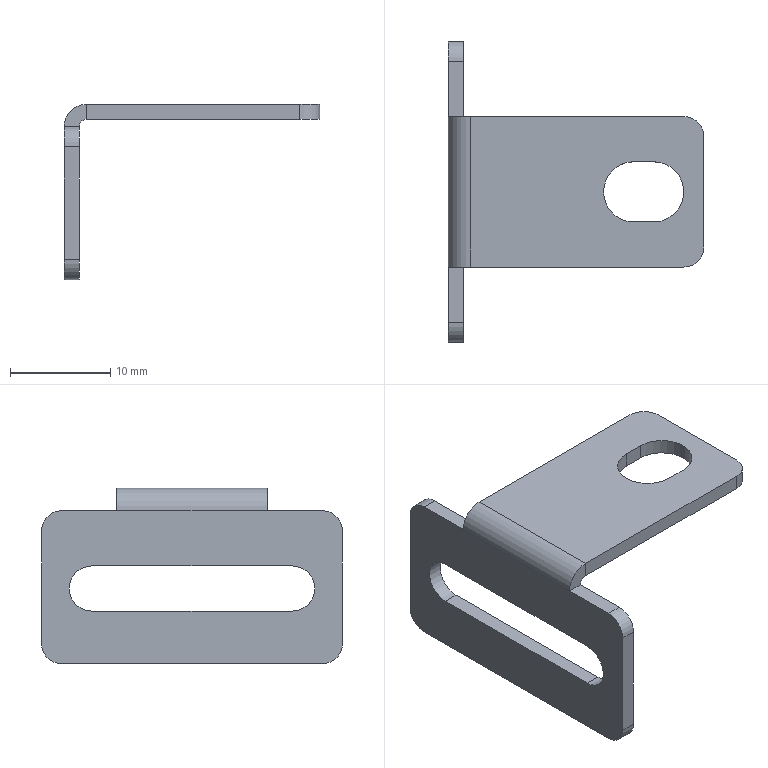Part | STEP file | H_ND24021-01-JG-029-BJ | 1 solid | 31 faces | box 25.5 x 30 x 17.5 mm | volume 1036 mm3 | plane 18 | cylinder 13 | commonest cylinder face diameters 4 x6 6 x3 4.5 x2 1.473 x1 4.473 x1